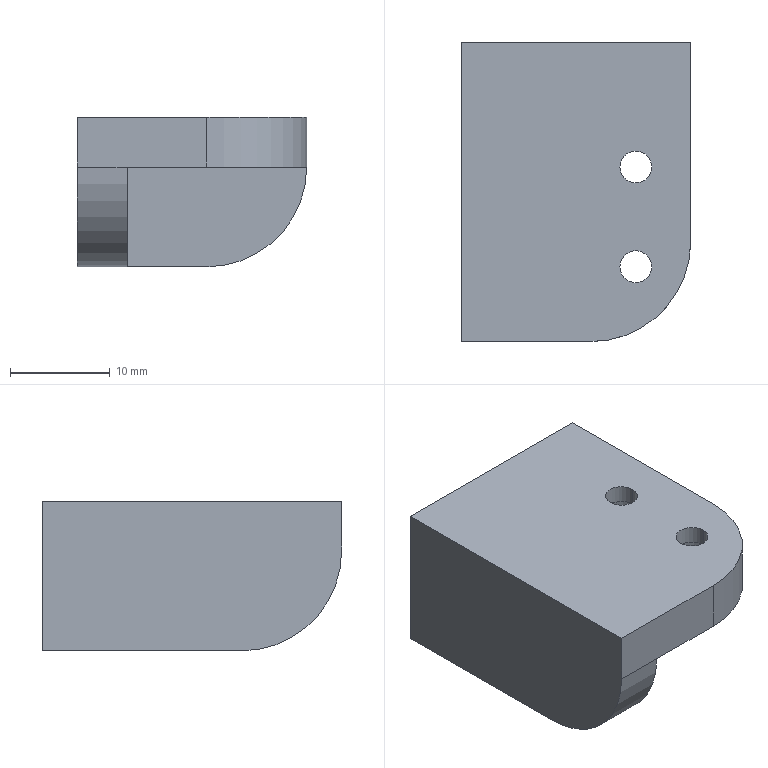Part | SolidWorks | features ICE 3, MoveFace 2, Extrusion 1, Fillet 1 | 1 solid | 22 faces | box 23 x 30 x 15 mm | volume 5306 mm3 | cylinder 11 | plane 11 | commonest cylinder face diameters 3.2 x4 6.2 x4 20 x3
STEP:
#1=CARTESIAN_POINT('',(18.1,7.5,15.7));
#2=VERTEX_POINT('',#1);
#3=CARTESIAN_POINT('',(11.9,7.5,15.7));
#4=VERTEX_POINT('',#3);
#5=CARTESIAN_POINT('',(15.,7.5,15.7));
#6=DIRECTION('',(0.,0.,-1.));
#7=DIRECTION('',(-1.,0.,0.));
#8=AXIS2_PLACEMENT_3D('',#5,#6,#7);
#9=CIRCLE('',#8,3.1);
#10=EDGE_CURVE('',#2,#4,#9,.T.);
#11=ORIENTED_EDGE('',*,*,#10,.F.);
#12=CARTESIAN_POINT('',(18.1,7.5,12.5));
#13=VERTEX_POINT('',#12);
#14=CARTESIAN_POINT('',(18.1,7.5,15.7));
#15=DIRECTION('',(0.,0.,-1.));
#16=VECTOR('',#15,1000.);
#17=LINE('',#14,#16);
#18=EDGE_CURVE('',#2,#13,#17,.T.);
#19=ORIENTED_EDGE('',*,*,#18,.T.);
#20=CARTESIAN_POINT('',(11.9,7.5,12.5));
#21=VERTEX_POINT('',#20);
#22=CARTESIAN_POINT('',(15.,7.5,12.5));
#23=DIRECTION('',(0.,0.,-1.));
#24=DIRECTION('',(-1.,0.,0.));
#25=AXIS2_PLACEMENT_3D('',#22,#23,#24);
#26=CIRCLE('',#25,3.1);
#27=EDGE_CURVE('',#13,#21,#26,.T.);
#28=ORIENTED_EDGE('',*,*,#27,.T.);
#29=CARTESIAN_POINT('',(11.9,7.5,15.7));
#30=DIRECTION('',(0.,0.,-1.));
#31=VECTOR('',#30,1000.);
#32=LINE('',#29,#31);
#33=EDGE_CURVE('',#4,#21,#32,.T.);
#34=ORIENTED_EDGE('',*,*,#33,.F.);
#35=EDGE_LOOP('',(#11,#19,#28,#34));
#36=FACE_OUTER_BOUND('',#35,.T.);
#37=CARTESIAN_POINT('',(15.,7.5,15.7));
#38=DIRECTION('',(0.,0.,-1.));
#39=DIRECTION('',(-1.,0.,0.));
#40=AXIS2_PLACEMENT_3D('',#37,#38,#39);
#41=CYLINDRICAL_SURFACE('',#40,3.1);
#42=ADVANCED_FACE('',(#36),#41,.F.);
#43=CARTESIAN_POINT('',(18.1,17.5,15.7));
#44=VERTEX_POINT('',#43);
#45=CARTESIAN_POINT('',(11.9,17.5,15.7));
#46=VERTEX_POINT('',#45);
#47=CARTESIAN_POINT('',(15.,17.5,15.7));
#48=DIRECTION('',(0.,0.,-1.));
#49=DIRECTION('',(-1.,0.,0.));
#50=AXIS2_PLACEMENT_3D('',#47,#48,#49);
#51=CIRCLE('',#50,3.1);
#52=EDGE_CURVE('',#44,#46,#51,.T.);
#53=ORIENTED_EDGE('',*,*,#52,.F.);
#54=CARTESIAN_POINT('',(18.1,17.5,12.5));
#55=VERTEX_POINT('',#54);
#56=CARTESIAN_POINT('',(18.1,17.5,15.7));
#57=DIRECTION('',(0.,0.,-1.));
#58=VECTOR('',#57,1000.);
#59=LINE('',#56,#58);
#60=EDGE_CURVE('',#44,#55,#59,.T.);
#61=ORIENTED_EDGE('',*,*,#60,.T.);
#62=CARTESIAN_POINT('',(11.9,17.5,12.5));
#63=VERTEX_POINT('',#62);
#64=CARTESIAN_POINT('',(15.,17.5,12.5));
#65=DIRECTION('',(0.,0.,-1.));
#66=DIRECTION('',(-1.,0.,0.));
#67=AXIS2_PLACEMENT_3D('',#64,#65,#66);
#68=CIRCLE('',#67,3.1);
#69=EDGE_CURVE('',#55,#63,#68,.T.);
#70=ORIENTED_EDGE('',*,*,#69,.T.);
#71=CARTESIAN_POINT('',(11.9,17.5,15.7));
#72=DIRECTION('',(0.,0.,-1.));
#73=VECTOR('',#72,1000.);
#74=LINE('',#71,#73);
#75=EDGE_CURVE('',#46,#63,#74,.T.);
#76=ORIENTED_EDGE('',*,*,#75,.F.);
#77=EDGE_LOOP('',(#53,#61,#70,#76));
#78=FACE_OUTER_BOUND('',#77,.T.);
#79=CARTESIAN_POINT('',(15.,17.5,15.7));
#80=DIRECTION('',(0.,0.,-1.));
#81=DIRECTION('',(-1.,0.,0.));
#82=AXIS2_PLACEMENT_3D('',#79,#80,#81);
#83=CYLINDRICAL_SURFACE('',#82,3.1);
#84=ADVANCED_FACE('',(#78),#83,.F.);
#85=CARTESIAN_POINT('',(16.6,17.5,17.5));
#86=VERTEX_POINT('',#85);
#87=CARTESIAN_POINT('',(13.4,17.5,17.5));
#88=VERTEX_POINT('',#87);
#89=CARTESIAN_POINT('',(15.,17.5,17.5));
#90=DIRECTION('',(0.,0.,-1.));
#91=DIRECTION('',(-1.,0.,0.));
#92=AXIS2_PLACEMENT_3D('',#89,#90,#91);
#93=CIRCLE('',#92,1.6);
#94=EDGE_CURVE('',#86,#88,#93,.T.);
#95=ORIENTED_EDGE('',*,*,#94,.F.);
#96=CARTESIAN_POINT('',(16.6,17.5,15.7));
#97=VERTEX_POINT('',#96);
#98=CARTESIAN_POINT('',(16.6,17.5,17.5));
#99=DIRECTION('',(0.,0.,-1.));
#100=VECTOR('',#99,1000.);
#101=LINE('',#98,#100);
#102=EDGE_CURVE('',#86,#97,#101,.T.);
#103=ORIENTED_EDGE('',*,*,#102,.T.);
#104=CARTESIAN_POINT('',(13.4,17.5,15.7));
#105=VERTEX_POINT('',#104);
#106=CARTESIAN_POINT('',(15.,17.5,15.7));
#107=DIRECTION('',(0.,0.,1.));
#108=DIRECTION('',(-1.,0.,0.));
#109=AXIS2_PLACEMENT_3D('',#106,#107,#108);
#110=CIRCLE('',#109,1.6);
#111=EDGE_CURVE('',#105,#97,#110,.T.);
#112=ORIENTED_EDGE('',*,*,#111,.F.);
#113=CARTESIAN_POINT('',(13.4,17.5,17.5));
#114=DIRECTION('',(0.,0.,-1.));
#115=VECTOR('',#114,1000.);
#116=LINE('',#113,#115);
#117=EDGE_CURVE('',#88,#105,#116,.T.);
#118=ORIENTED_EDGE('',*,*,#117,.F.);
#119=EDGE_LOOP('',(#95,#103,#112,#118));
#120=FACE_OUTER_BOUND('',#119,.T.);
#121=CARTESIAN_POINT('',(15.,17.5,17.5));
#122=DIRECTION('',(0.,0.,-1.));
#123=DIRECTION('',(-1.,0.,0.));
#124=AXIS2_PLACEMENT_3D('',#121,#122,#123);
#125=CYLINDRICAL_SURFACE('',#124,1.6);
#126=ADVANCED_FACE('',(#120),#125,.F.);
#127=CARTESIAN_POINT('',(16.6,7.5,17.5));
#128=VERTEX_POINT('',#127);
#129=CARTESIAN_POINT('',(13.4,7.5,17.5));
#130=VERTEX_POINT('',#129);
#131=CARTESIAN_POINT('',(15.,7.5,17.5));
#132=DIRECTION('',(0.,0.,-1.));
#133=DIRECTION('',(-1.,0.,0.));
#134=AXIS2_PLACEMENT_3D('',#131,#132,#133);
#135=CIRCLE('',#134,1.6);
#136=EDGE_CURVE('',#128,#130,#135,.T.);
#137=ORIENTED_EDGE('',*,*,#136,.F.);
#138=CARTESIAN_POINT('',(16.6,7.5,15.7));
#139=VERTEX_POINT('',#138);
#140=CARTESIAN_POINT('',(16.6,7.5,17.5));
#141=DIRECTION('',(0.,0.,-1.));
#142=VECTOR('',#141,1000.);
#143=LINE('',#140,#142);
#144=EDGE_CURVE('',#128,#139,#143,.T.);
#145=ORIENTED_EDGE('',*,*,#144,.T.);
#146=CARTESIAN_POINT('',(13.4,7.5,15.7));
#147=VERTEX_POINT('',#146);
#148=CARTESIAN_POINT('',(15.,7.5,15.7));
#149=DIRECTION('',(0.,0.,1.));
#150=DIRECTION('',(-1.,0.,0.));
#151=AXIS2_PLACEMENT_3D('',#148,#149,#150);
#152=CIRCLE('',#151,1.6);
#153=EDGE_CURVE('',#147,#139,#152,.T.);
#154=ORIENTED_EDGE('',*,*,#153,.F.);
#155=CARTESIAN_POINT('',(13.4,7.5,17.5));
#156=DIRECTION('',(0.,0.,-1.));
#157=VECTOR('',#156,1000.);
#158=LINE('',#155,#157);
#159=EDGE_CURVE('',#130,#147,#158,.T.);
#160=ORIENTED_EDGE('',*,*,#159,.F.);
#161=EDGE_LOOP('',(#137,#145,#154,#160));
#162=FACE_OUTER_BOUND('',#161,.T.);
#163=CARTESIAN_POINT('',(15.,7.5,17.5));
#164=DIRECTION('',(0.,0.,-1.));
#165=DIRECTION('',(-1.,0.,0.));
#166=AXIS2_PLACEMENT_3D('',#163,#164,#165);
#167=CYLINDRICAL_SURFACE('',#166,1.6);
#168=ADVANCED_FACE('',(#162),#167,.F.);
#169=ORIENTED_EDGE('',*,*,#144,.F.);
#170=CARTESIAN_POINT('',(15.,7.5,17.5));
#171=DIRECTION('',(0.,0.,-1.));
#172=DIRECTION('',(-1.,0.,0.));
#173=AXIS2_PLACEMENT_3D('',#170,#171,#172);
#174=CIRCLE('',#173,1.6);
#175=EDGE_CURVE('',#130,#128,#174,.T.);
#176=ORIENTED_EDGE('',*,*,#175,.F.);
#177=ORIENTED_EDGE('',*,*,#159,.T.);
#178=CARTESIAN_POINT('',(15.,7.5,15.7));
#179=DIRECTION('',(0.,0.,1.));
#180=DIRECTION('',(-1.,0.,0.));
#181=AXIS2_PLACEMENT_3D('',#178,#179,#180);
#182=CIRCLE('',#181,1.6);
#183=EDGE_CURVE('',#139,#147,#182,.T.);
#184=ORIENTED_EDGE('',*,*,#183,.F.);
#185=EDGE_LOOP('',(#169,#176,#177,#184));
#186=FACE_OUTER_BOUND('',#185,.T.);
#187=CARTESIAN_POINT('',(15.,7.5,17.5));
#188=DIRECTION('',(0.,0.,-1.));
#189=DIRECTION('',(-1.,0.,0.));
#190=AXIS2_PLACEMENT_3D('',#187,#188,#189);
#191=CYLINDRICAL_SURFACE('',#190,1.6);
#192=ADVANCED_FACE('',(#186),#191,.F.);
#193=ORIENTED_EDGE('',*,*,#102,.F.);
#194=CARTESIAN_POINT('',(15.,17.5,17.5));
#195=DIRECTION('',(0.,0.,-1.));
#196=DIRECTION('',(-1.,0.,0.));
#197=AXIS2_PLACEMENT_3D('',#194,#195,#196);
#198=CIRCLE('',#197,1.6);
#199=EDGE_CURVE('',#88,#86,#198,.T.);
#200=ORIENTED_EDGE('',*,*,#199,.F.);
#201=ORIENTED_EDGE('',*,*,#117,.T.);
#202=CARTESIAN_POINT('',(15.,17.5,15.7));
#203=DIRECTION('',(0.,0.,1.));
#204=DIRECTION('',(-1.,0.,0.));
#205=AXIS2_PLACEMENT_3D('',#202,#203,#204);
#206=CIRCLE('',#205,1.6);
#207=EDGE_CURVE('',#97,#105,#206,.T.);
#208=ORIENTED_EDGE('',*,*,#207,.F.);
#209=EDGE_LOOP('',(#193,#200,#201,#208));
#210=FACE_OUTER_BOUND('',#209,.T.);
#211=CARTESIAN_POINT('',(15.,17.5,17.5));
#212=DIRECTION('',(0.,0.,-1.));
#213=DIRECTION('',(-1.,0.,0.));
#214=AXIS2_PLACEMENT_3D('',#211,#212,#213);
#215=CYLINDRICAL_SURFACE('',#214,1.6);
#216=ADVANCED_FACE('',(#210),#215,.F.);
#217=CARTESIAN_POINT('',(15.,7.5,12.5));
#218=DIRECTION('',(0.,0.,-1.));
#219=DIRECTION('',(-1.,0.,0.));
#220=AXIS2_PLACEMENT_3D('',#217,#218,#219);
#221=CIRCLE('',#220,3.1);
#222=EDGE_CURVE('',#21,#13,#221,.T.);
#223=ORIENTED_EDGE('',*,*,#222,.F.);
#224=ORIENTED_EDGE('',*,*,#27,.F.);
#225=EDGE_LOOP('',(#223,#224));
#226=FACE_BOUND('',#225,.T.);
#227=CARTESIAN_POINT('',(15.,17.5,12.5));
#228=DIRECTION('',(0.,0.,-1.));
#229=DIRECTION('',(-1.,0.,0.));
#230=AXIS2_PLACEMENT_3D('',#227,#228,#229);
#231=CIRCLE('',#230,3.1);
#232=EDGE_CURVE('',#63,#55,#231,.T.);
#233=ORIENTED_EDGE('',*,*,#232,.F.);
#234=ORIENTED_EDGE('',*,*,#69,.F.);
#235=EDGE_LOOP('',(#233,#234));
#236=FACE_BOUND('',#235,.T.);
#237=CARTESIAN_POINT('',(20.5,25.,12.5));
#238=VERTEX_POINT('',#237);
#239=CARTESIAN_POINT('',(20.5,10.,12.5));
#240=VERTEX_POINT('',#239);
#241=CARTESIAN_POINT('',(20.5,30.,12.5));
#242=DIRECTION('',(0.,-1.,0.));
#243=VECTOR('',#242,1000.);
#244=LINE('',#241,#243);
#245=EDGE_CURVE('',#238,#240,#244,.T.);
#246=ORIENTED_EDGE('',*,*,#245,.T.);
#247=CARTESIAN_POINT('',(10.5,0.,12.5));
#248=VERTEX_POINT('',#247);
#249=CARTESIAN_POINT('',(10.5,10.,12.5));
#250=DIRECTION('',(0.,0.,-1.));
#251=DIRECTION('',(-1.,0.,0.));
#252=AXIS2_PLACEMENT_3D('',#249,#250,#251);
#253=CIRCLE('',#252,10.);
#254=EDGE_CURVE('',#240,#248,#253,.T.);
#255=ORIENTED_EDGE('',*,*,#254,.T.);
#256=CARTESIAN_POINT('',(2.5,0.,12.5));
#257=VERTEX_POINT('',#256);
#258=CARTESIAN_POINT('',(0.,0.,12.5));
#259=DIRECTION('',(1.,0.,0.));
#260=VECTOR('',#259,1000.);
#261=LINE('',#258,#260);
#262=EDGE_CURVE('',#257,#248,#261,.T.);
#263=ORIENTED_EDGE('',*,*,#262,.F.);
#264=CARTESIAN_POINT('',(2.5,25.,12.5));
#265=VERTEX_POINT('',#264);
#266=CARTESIAN_POINT('',(2.5,30.,12.5));
#267=DIRECTION('',(0.,-1.,0.));
#268=VECTOR('',#267,1000.);
#269=LINE('',#266,#268);
#270=EDGE_CURVE('',#265,#257,#269,.T.);
#271=ORIENTED_EDGE('',*,*,#270,.F.);
#272=CARTESIAN_POINT('',(0.,25.,12.5));
#273=DIRECTION('',(1.,0.,0.));
#274=VECTOR('',#273,1000.);
#275=LINE('',#272,#274);
#276=EDGE_CURVE('',#265,#238,#275,.T.);
#277=ORIENTED_EDGE('',*,*,#276,.T.);
#278=EDGE_LOOP('',(#246,#255,#263,#271,#277));
#279=FACE_OUTER_BOUND('',#278,.T.);
#280=CARTESIAN_POINT('',(0.,30.,12.5));
#281=DIRECTION('',(0.,0.,-1.));
#282=DIRECTION('',(-1.,0.,0.));
#283=AXIS2_PLACEMENT_3D('',#280,#281,#282);
#284=PLANE('',#283);
#285=ADVANCED_FACE('',(#226,#236,#279),#284,.T.);
#286=ORIENTED_EDGE('',*,*,#270,.T.);
#287=CARTESIAN_POINT('',(2.5,10.,2.5));
#288=VERTEX_POINT('',#287);
#289=CARTESIAN_POINT('',(2.5,10.,12.5));
#290=DIRECTION('',(1.,0.,0.));
#291=DIRECTION('',(0.,0.,1.));
#292=AXIS2_PLACEMENT_3D('',#289,#290,#291);
#293=CIRCLE('',#292,10.);
#294=EDGE_CURVE('',#257,#288,#293,.T.);
#295=ORIENTED_EDGE('',*,*,#294,.T.);
#296=CARTESIAN_POINT('',(2.5,25.,2.5));
#297=VERTEX_POINT('',#296);
#298=CARTESIAN_POINT('',(2.5,30.,2.5));
#299=DIRECTION('',(0.,-1.,0.));
#300=VECTOR('',#299,1000.);
#301=LINE('',#298,#300);
#302=EDGE_CURVE('',#297,#288,#301,.T.);
#303=ORIENTED_EDGE('',*,*,#302,.F.);
#304=CARTESIAN_POINT('',(2.5,25.,0.));
#305=DIRECTION('',(0.,0.,-1.));
#306=VECTOR('',#305,1000.);
#307=LINE('',#304,#306);
#308=EDGE_CURVE('',#265,#297,#307,.T.);
#309=ORIENTED_EDGE('',*,*,#308,.F.);
#310=EDGE_LOOP('',(#286,#295,#303,#309));
#311=FACE_OUTER_BOUND('',#310,.T.);
#312=CARTESIAN_POINT('',(2.5,30.,0.));
#313=DIRECTION('',(-1.,0.,0.));
#314=DIRECTION('',(0.,0.,1.));
#315=AXIS2_PLACEMENT_3D('',#312,#313,#314);
#316=PLANE('',#315);
#317=ADVANCED_FACE('',(#311),#316,.F.);
#318=CARTESIAN_POINT('',(20.5,30.,17.5));
#319=VERTEX_POINT('',#318);
#320=CARTESIAN_POINT('',(20.5,10.,17.5));
#321=VERTEX_POINT('',#320);
#322=CARTESIAN_POINT('',(20.5,30.,17.5));
#323=DIRECTION('',(0.,-1.,0.));
#324=VECTOR('',#323,1000.);
#325=LINE('',#322,#324);
#326=EDGE_CURVE('',#319,#321,#325,.T.);
#327=ORIENTED_EDGE('',*,*,#326,.T.);
#328=CARTESIAN_POINT('',(20.5,10.,12.5));
#329=DIRECTION('',(0.,0.,-1.));
#330=VECTOR('',#329,1000.);
#331=LINE('',#328,#330);
#332=EDGE_CURVE('',#321,#240,#331,.T.);
#333=ORIENTED_EDGE('',*,*,#332,.T.);
#334=ORIENTED_EDGE('',*,*,#245,.F.);
#335=CARTESIAN_POINT('',(20.5,30.,12.5));
#336=VERTEX_POINT('',#335);
#337=CARTESIAN_POINT('',(20.5,30.,12.5));
#338=DIRECTION('',(0.,1.,0.));
#339=VECTOR('',#338,1000.);
#340=LINE('',#337,#339);
#341=EDGE_CURVE('',#238,#336,#340,.T.);
#342=ORIENTED_EDGE('',*,*,#341,.T.);
#343=CARTESIAN_POINT('',(20.5,30.,0.));
#344=DIRECTION('',(0.,0.,1.));
#345=VECTOR('',#344,1000.);
#346=LINE('',#343,#345);
#347=EDGE_CURVE('',#336,#319,#346,.T.);
#348=ORIENTED_EDGE('',*,*,#347,.T.);
#349=EDGE_LOOP('',(#327,#333,#334,#342,#348));
#350=FACE_OUTER_BOUND('',#349,.T.);
#351=CARTESIAN_POINT('',(20.5,30.,0.));
#352=DIRECTION('',(1.,0.,0.));
#353=DIRECTION('',(0.,0.,-1.));
#354=AXIS2_PLACEMENT_3D('',#351,#352,#353);
#355=PLANE('',#354);
#356=ADVANCED_FACE('',(#350),#355,.T.);
#357=CARTESIAN_POINT('',(-2.5,30.,2.5));
#358=VERTEX_POINT('',#357);
#359=CARTESIAN_POINT('',(10.5,30.,2.5));
#360=VERTEX_POINT('',#359);
#361=CARTESIAN_POINT('',(0.,30.,2.5));
#362=DIRECTION('',(1.,0.,0.));
#363=VECTOR('',#362,1000.);
#364=LINE('',#361,#363);
#365=EDGE_CURVE('',#358,#360,#364,.T.);
#366=ORIENTED_EDGE('',*,*,#365,.T.);
#367=CARTESIAN_POINT('',(10.5,25.,2.5));
#368=VERTEX_POINT('',#367);
#369=CARTESIAN_POINT('',(10.5,30.,2.5));
#370=DIRECTION('',(0.,-1.,0.));
#371=VECTOR('',#370,1000.);
#372=LINE('',#369,#371);
#373=EDGE_CURVE('',#360,#368,#372,.T.);
#374=ORIENTED_EDGE('',*,*,#373,.T.);
#375=CARTESIAN_POINT('',(-2.5,25.,2.5));
#376=DIRECTION('',(-1.,0.,0.));
#377=VECTOR('',#376,1000.);
#378=LINE('',#375,#377);
#379=EDGE_CURVE('',#368,#297,#378,.T.);
#380=ORIENTED_EDGE('',*,*,#379,.T.);
#381=ORIENTED_EDGE('',*,*,#302,.T.);
#382=CARTESIAN_POINT('',(-2.5,10.,2.5));
#383=VERTEX_POINT('',#382);
#384=CARTESIAN_POINT('',(-2.5,10.,2.5));
#385=DIRECTION('',(-1.,0.,0.));
#386=VECTOR('',#385,1000.);
#387=LINE('',#384,#386);
#388=EDGE_CURVE('',#288,#383,#387,.T.);
#389=ORIENTED_EDGE('',*,*,#388,.T.);
#390=CARTESIAN_POINT('',(-2.5,30.,2.5));
#391=DIRECTION('',(0.,-1.,0.));
#392=VECTOR('',#391,1000.);
#393=LINE('',#390,#392);
#394=EDGE_CURVE('',#358,#383,#393,.T.);
#395=ORIENTED_EDGE('',*,*,#394,.F.);
#396=EDGE_LOOP('',(#366,#374,#380,#381,#389,#395));
#397=FACE_OUTER_BOUND('',#396,.T.);
#398=CARTESIAN_POINT('',(0.,30.,2.5));
#399=DIRECTION('',(0.,0.,-1.));
#400=DIRECTION('',(-1.,0.,0.));
#401=AXIS2_PLACEMENT_3D('',#398,#399,#400);
#402=PLANE('',#401);
#403=ADVANCED_FACE('',(#397),#402,.T.);
#404=ORIENTED_EDGE('',*,*,#394,.T.);
#405=CARTESIAN_POINT('',(-2.5,0.,12.5));
#406=VERTEX_POINT('',#405);
#407=CARTESIAN_POINT('',(-2.5,10.,12.5));
#408=DIRECTION('',(-1.,0.,0.));
#409=DIRECTION('',(0.,0.,1.));
#410=AXIS2_PLACEMENT_3D('',#407,#408,#409);
#411=CIRCLE('',#410,10.);
#412=EDGE_CURVE('',#383,#406,#411,.T.);
#413=ORIENTED_EDGE('',*,*,#412,.T.);
#414=CARTESIAN_POINT('',(-2.5,0.,17.5));
#415=VERTEX_POINT('',#414);
#416=CARTESIAN_POINT('',(-2.5,0.,0.));
#417=DIRECTION('',(0.,0.,-1.));
#418=VECTOR('',#417,1000.);
#419=LINE('',#416,#418);
#420=EDGE_CURVE('',#415,#406,#419,.T.);
#421=ORIENTED_EDGE('',*,*,#420,.F.);
#422=CARTESIAN_POINT('',(-2.5,30.,17.5));
#423=VERTEX_POINT('',#422);
#424=CARTESIAN_POINT('',(-2.5,30.,17.5));
#425=DIRECTION('',(0.,-1.,0.));
#426=VECTOR('',#425,1000.);
#427=LINE('',#424,#426);
#428=EDGE_CURVE('',#423,#415,#427,.T.);
#429=ORIENTED_EDGE('',*,*,#428,.F.);
#430=CARTESIAN_POINT('',(-2.5,30.,0.));
#431=DIRECTION('',(0.,0.,-1.));
#432=VECTOR('',#431,1000.);
#433=LINE('',#430,#432);
#434=EDGE_CURVE('',#423,#358,#433,.T.);
#435=ORIENTED_EDGE('',*,*,#434,.T.);
#436=EDGE_LOOP('',(#404,#413,#421,#429,#435));
#437=FACE_OUTER_BOUND('',#436,.T.);
#438=CARTESIAN_POINT('',(-2.5,30.,0.));
#439=DIRECTION('',(-1.,0.,0.));
#440=DIRECTION('',(0.,0.,1.));
#441=AXIS2_PLACEMENT_3D('',#438,#439,#440);
#442=PLANE('',#441);
#443=ADVANCED_FACE('',(#437),#442,.T.);
#444=ORIENTED_EDGE('',*,*,#199,.T.);
#445=ORIENTED_EDGE('',*,*,#94,.T.);
#446=EDGE_LOOP('',(#444,#445));
#447=FACE_BOUND('',#446,.T.);
#448=ORIENTED_EDGE('',*,*,#175,.T.);
#449=ORIENTED_EDGE('',*,*,#136,.T.);
#450=EDGE_LOOP('',(#448,#449));
#451=FACE_BOUND('',#450,.T.);
#452=CARTESIAN_POINT('',(10.5,0.,17.5));
#453=VERTEX_POINT('',#452);
#454=CARTESIAN_POINT('',(0.,0.,17.5));
#455=DIRECTION('',(1.,0.,0.));
#456=VECTOR('',#455,1000.);
#457=LINE('',#454,#456);
#458=EDGE_CURVE('',#415,#453,#457,.T.);
#459=ORIENTED_EDGE('',*,*,#458,.T.);
#460=CARTESIAN_POINT('',(10.5,10.,17.5));
#461=DIRECTION('',(0.,0.,1.));
#462=DIRECTION('',(-1.,0.,0.));
#463=AXIS2_PLACEMENT_3D('',#460,#461,#462);
#464=CIRCLE('',#463,10.);
#465=EDGE_CURVE('',#453,#321,#464,.T.);
#466=ORIENTED_EDGE('',*,*,#465,.T.);
#467=ORIENTED_EDGE('',*,*,#326,.F.);
#468=CARTESIAN_POINT('',(0.,30.,17.5));
#469=DIRECTION('',(1.,0.,0.));
#470=VECTOR('',#469,1000.);
#471=LINE('',#468,#470);
#472=EDGE_CURVE('',#423,#319,#471,.T.);
#473=ORIENTED_EDGE('',*,*,#472,.F.);
#474=ORIENTED_EDGE('',*,*,#428,.T.);
#475=EDGE_LOOP('',(#459,#466,#467,#473,#474));
#476=FACE_OUTER_BOUND('',#475,.T.);
#477=CARTESIAN_POINT('',(0.,30.,17.5));
#478=DIRECTION('',(0.,0.,-1.));
#479=DIRECTION('',(-1.,0.,0.));
#480=AXIS2_PLACEMENT_3D('',#477,#478,#479);
#481=PLANE('',#480);
#482=ADVANCED_FACE('',(#447,#451,#476),#481,.F.);
#483=ORIENTED_EDGE('',*,*,#347,.F.);
#484=CARTESIAN_POINT('',(10.5,30.,12.5));
#485=DIRECTION('',(0.,1.,0.));
#486=DIRECTION('',(0.,0.,1.));
#487=AXIS2_PLACEMENT_3D('',#484,#485,#486);
#488=CIRCLE('',#487,10.);
#489=EDGE_CURVE('',#336,#360,#488,.T.);
#490=ORIENTED_EDGE('',*,*,#489,.T.);
#491=ORIENTED_EDGE('',*,*,#365,.F.);
#492=ORIENTED_EDGE('',*,*,#434,.F.);
#493=ORIENTED_EDGE('',*,*,#472,.T.);
#494=EDGE_LOOP('',(#483,#490,#491,#492,#493));
#495=FACE_OUTER_BOUND('',#494,.T.);
#496=CARTESIAN_POINT('',(0.,30.,0.));
#497=DIRECTION('',(0.,1.,0.));
#498=DIRECTION('',(0.,0.,1.));
#499=AXIS2_PLACEMENT_3D('',#496,#497,#498);
#500=PLANE('',#499);
#501=ADVANCED_FACE('',(#495),#500,.T.);
#502=ORIENTED_EDGE('',*,*,#262,.T.);
#503=CARTESIAN_POINT('',(10.5,0.,17.5));
#504=DIRECTION('',(0.,0.,1.));
#505=VECTOR('',#504,1000.);
#506=LINE('',#503,#505);
#507=EDGE_CURVE('',#248,#453,#506,.T.);
#508=ORIENTED_EDGE('',*,*,#507,.T.);
#509=ORIENTED_EDGE('',*,*,#458,.F.);
#510=ORIENTED_EDGE('',*,*,#420,.T.);
#511=CARTESIAN_POINT('',(2.5,0.,12.5));
#512=DIRECTION('',(1.,0.,0.));
#513=VECTOR('',#512,1000.);
#514=LINE('',#511,#513);
#515=EDGE_CURVE('',#406,#257,#514,.T.);
#516=ORIENTED_EDGE('',*,*,#515,.T.);
#517=EDGE_LOOP('',(#502,#508,#509,#510,#516));
#518=FACE_OUTER_BOUND('',#517,.T.);
#519=CARTESIAN_POINT('',(0.,0.,0.));
#520=DIRECTION('',(0.,1.,0.));
#521=DIRECTION('',(0.,0.,1.));
#522=AXIS2_PLACEMENT_3D('',#519,#520,#521);
#523=PLANE('',#522);
#524=ADVANCED_FACE('',(#518),#523,.F.);
#525=ORIENTED_EDGE('',*,*,#379,.F.);
#526=CARTESIAN_POINT('',(10.5,25.,12.5));
#527=DIRECTION('',(0.,-1.,0.));
#528=DIRECTION('',(0.,0.,1.));
#529=AXIS2_PLACEMENT_3D('',#526,#527,#528);
#530=CIRCLE('',#529,10.);
#531=EDGE_CURVE('',#368,#238,#530,.T.);
#532=ORIENTED_EDGE('',*,*,#531,.T.);
#533=ORIENTED_EDGE('',*,*,#276,.F.);
#534=ORIENTED_EDGE('',*,*,#308,.T.);
#535=EDGE_LOOP('',(#525,#532,#533,#534));
#536=FACE_OUTER_BOUND('',#535,.T.);
#537=CARTESIAN_POINT('',(0.,25.,0.));
#538=DIRECTION('',(0.,1.,0.));
#539=DIRECTION('',(0.,0.,1.));
#540=AXIS2_PLACEMENT_3D('',#537,#538,#539);
#541=PLANE('',#540);
#542=ADVANCED_FACE('',(#536),#541,.F.);
#543=CARTESIAN_POINT('',(15.,17.5,15.7));
#544=DIRECTION('',(0.,0.,-1.));
#545=DIRECTION('',(-1.,0.,0.));
#546=AXIS2_PLACEMENT_3D('',#543,#544,#545);
#547=CIRCLE('',#546,3.1);
#548=EDGE_CURVE('',#46,#44,#547,.T.);
#549=ORIENTED_EDGE('',*,*,#548,.T.);
#550=ORIENTED_EDGE('',*,*,#52,.T.);
#551=EDGE_LOOP('',(#549,#550));
#552=FACE_OUTER_BOUND('',#551,.T.);
#553=ORIENTED_EDGE('',*,*,#111,.T.);
#554=ORIENTED_EDGE('',*,*,#207,.T.);
#555=EDGE_LOOP('',(#553,#554));
#556=FACE_BOUND('',#555,.T.);
#557=CARTESIAN_POINT('',(15.,17.5,15.7));
#558=DIRECTION('',(0.,0.,-1.));
#559=DIRECTION('',(-1.,0.,0.));
#560=AXIS2_PLACEMENT_3D('',#557,#558,#559);
#561=PLANE('',#560);
#562=ADVANCED_FACE('',(#552,#556),#561,.T.);
#563=ORIENTED_EDGE('',*,*,#60,.F.);
#564=ORIENTED_EDGE('',*,*,#548,.F.);
#565=ORIENTED_EDGE('',*,*,#75,.T.);
#566=ORIENTED_EDGE('',*,*,#232,.T.);
#567=EDGE_LOOP('',(#563,#564,#565,#566));
#568=FACE_OUTER_BOUND('',#567,.T.);
#569=CARTESIAN_POINT('',(15.,17.5,15.7));
#570=DIRECTION('',(0.,0.,-1.));
#571=DIRECTION('',(-1.,0.,0.));
#572=AXIS2_PLACEMENT_3D('',#569,#570,#571);
#573=CYLINDRICAL_SURFACE('',#572,3.1);
#574=ADVANCED_FACE('',(#568),#573,.F.);
#575=CARTESIAN_POINT('',(15.,7.5,15.7));
#576=DIRECTION('',(0.,0.,-1.));
#577=DIRECTION('',(-1.,0.,0.));
#578=AXIS2_PLACEMENT_3D('',#575,#576,#577);
#579=CIRCLE('',#578,3.1);
#580=EDGE_CURVE('',#4,#2,#579,.T.);
#581=ORIENTED_EDGE('',*,*,#580,.T.);
#582=ORIENTED_EDGE('',*,*,#10,.T.);
#583=EDGE_LOOP('',(#581,#582));
#584=FACE_OUTER_BOUND('',#583,.T.);
#585=ORIENTED_EDGE('',*,*,#153,.T.);
#586=ORIENTED_EDGE('',*,*,#183,.T.);
#587=EDGE_LOOP('',(#585,#586));
#588=FACE_BOUND('',#587,.T.);
#589=CARTESIAN_POINT('',(15.,7.5,15.7));
#590=DIRECTION('',(0.,0.,-1.));
#591=DIRECTION('',(-1.,0.,0.));
#592=AXIS2_PLACEMENT_3D('',#589,#590,#591);
#593=PLANE('',#592);
#594=ADVANCED_FACE('',(#584,#588),#593,.T.);
#595=ORIENTED_EDGE('',*,*,#18,.F.);
#596=ORIENTED_EDGE('',*,*,#580,.F.);
#597=ORIENTED_EDGE('',*,*,#33,.T.);
#598=ORIENTED_EDGE('',*,*,#222,.T.);
#599=EDGE_LOOP('',(#595,#596,#597,#598));
#600=FACE_OUTER_BOUND('',#599,.T.);
#601=CARTESIAN_POINT('',(15.,7.5,15.7));
#602=DIRECTION('',(0.,0.,-1.));
#603=DIRECTION('',(-1.,0.,0.));
#604=AXIS2_PLACEMENT_3D('',#601,#602,#603);
#605=CYLINDRICAL_SURFACE('',#604,3.1);
#606=ADVANCED_FACE('',(#600),#605,.F.);
#607=ORIENTED_EDGE('',*,*,#254,.F.);
#608=ORIENTED_EDGE('',*,*,#332,.F.);
#609=ORIENTED_EDGE('',*,*,#465,.F.);
#610=ORIENTED_EDGE('',*,*,#507,.F.);
#611=EDGE_LOOP('',(#607,#608,#609,#610));
#612=FACE_OUTER_BOUND('',#611,.T.);
#613=CARTESIAN_POINT('',(10.5,10.,0.));
#614=DIRECTION('',(0.,0.,-1.));
#615=DIRECTION('',(-1.,0.,0.));
#616=AXIS2_PLACEMENT_3D('',#613,#614,#615);
#617=CYLINDRICAL_SURFACE('',#616,10.);
#618=ADVANCED_FACE('',(#612),#617,.T.);
#619=ORIENTED_EDGE('',*,*,#531,.F.);
#620=ORIENTED_EDGE('',*,*,#373,.F.);
#621=ORIENTED_EDGE('',*,*,#489,.F.);
#622=ORIENTED_EDGE('',*,*,#341,.F.);
#623=EDGE_LOOP('',(#619,#620,#621,#622));
#624=FACE_OUTER_BOUND('',#623,.T.);
#625=CARTESIAN_POINT('',(10.5,30.,12.5));
#626=DIRECTION('',(0.,1.,0.));
#627=DIRECTION('',(0.,0.,1.));
#628=AXIS2_PLACEMENT_3D('',#625,#626,#627);
#629=CYLINDRICAL_SURFACE('',#628,10.);
#630=ADVANCED_FACE('',(#624),#629,.T.);
#631=ORIENTED_EDGE('',*,*,#412,.F.);
#632=ORIENTED_EDGE('',*,*,#388,.F.);
#633=ORIENTED_EDGE('',*,*,#294,.F.);
#634=ORIENTED_EDGE('',*,*,#515,.F.);
#635=EDGE_LOOP('',(#631,#632,#633,#634));
#636=FACE_OUTER_BOUND('',#635,.T.);
#637=CARTESIAN_POINT('',(0.,10.,12.5));
#638=DIRECTION('',(-1.,0.,0.));
#639=DIRECTION('',(0.,0.,1.));
#640=AXIS2_PLACEMENT_3D('',#637,#638,#639);
#641=CYLINDRICAL_SURFACE('',#640,10.);
#642=ADVANCED_FACE('',(#636),#641,.T.);
#643=CLOSED_SHELL('',(#42,#84,#126,#168,#192,#216,#285,#317,#356,#403,#443,#482,#501,#524,#542,#562,#574,#594,#606,#618,#630,#642));
#644=MANIFOLD_SOLID_BREP('',#643);
#645=CARTESIAN_POINT('',(0.,0.,0.));
#646=DIRECTION('',(0.,0.,1.));
#647=DIRECTION('',(1.,0.,0.));
#648=AXIS2_PLACEMENT_3D('',#645,#646,#647);
#649=(LENGTH_UNIT()NAMED_UNIT(*)SI_UNIT(.MILLI.,.METRE.));
#650=UNCERTAINTY_MEASURE_WITH_UNIT(LENGTH_MEASURE(0.00001),#649,'','');
#651=(NAMED_UNIT(*)PLANE_ANGLE_UNIT()SI_UNIT($,.RADIAN.));
#652=(NAMED_UNIT(*)SI_UNIT($,.STERADIAN.)SOLID_ANGLE_UNIT());
#653=(GEOMETRIC_REPRESENTATION_CONTEXT(3)GLOBAL_UNCERTAINTY_ASSIGNED_CONTEXT((#650))GLOBAL_UNIT_ASSIGNED_CONTEXT((#649,#651,#652))REPRESENTATION_CONTEXT('',''));
#654=ADVANCED_BREP_SHAPE_REPRESENTATION('',(#644,#648),#653);